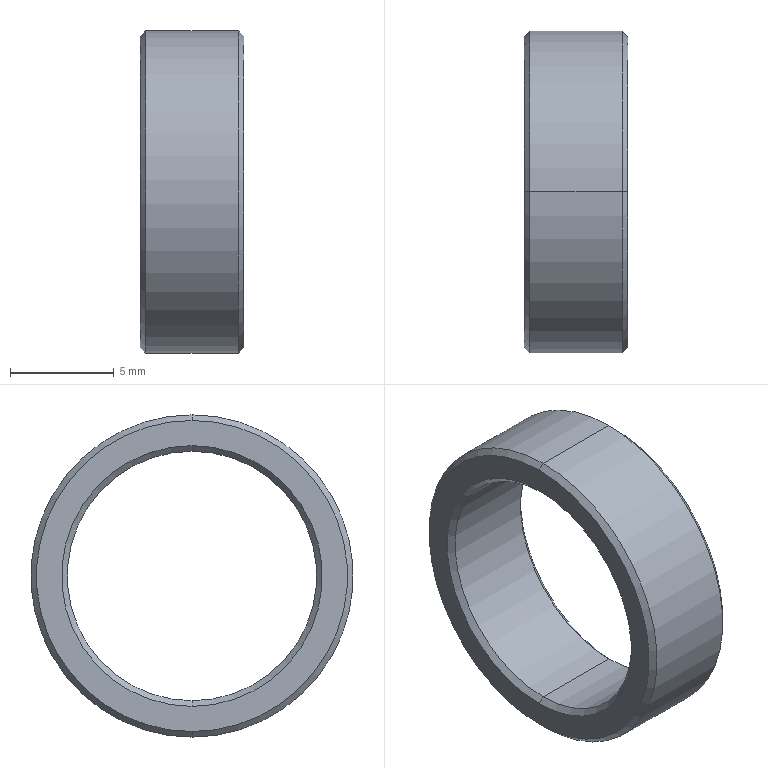Part | STEP file | GELIHUAN15-5-12-1 | 1 solid | 14 faces | box 5 x 15.5 x 15.5 mm | volume 371.674 mm3 | cone 8 | cylinder 4 | plane 2 | commonest cylinder face diameters 12 x2 15.5 x2
STEP:
#1=CARTESIAN_POINT('',(0.,0.,0.));
#2=DIRECTION('',(0.,0.,1.));
#3=DIRECTION('',(1.,0.,0.));
#4=AXIS2_PLACEMENT_3D('',#1,#2,#3);
#5=CARTESIAN_POINT('',(-8.965,58.327,-47.206));
#6=VERTEX_POINT('',#5);
#7=CARTESIAN_POINT('',(-4.505,58.327,-47.206));
#8=VERTEX_POINT('',#7);
#9=CARTESIAN_POINT('',(-8.965,58.327,-47.206));
#10=DIRECTION('',(1.,0.,0.));
#11=VECTOR('',#10,1.);
#12=LINE('',#9,#11);
#13=CARTESIAN_POINT('',(-8.965,58.327,-41.206));
#14=DIRECTION('',(1.,0.,0.));
#15=DIRECTION('',(0.,0.,-1.));
#16=AXIS2_PLACEMENT_3D('',#13,#14,#15);
#17=CYLINDRICAL_SURFACE('',#16,6.);
#18=CARTESIAN_POINT('',(6.283,0.));
#19=DIRECTION('',(0.,1.));
#20=VECTOR('',#19,1.);
#21=LINE('',#18,#20);
#22=(GEOMETRIC_REPRESENTATION_CONTEXT(2)PARAMETRIC_REPRESENTATION_CONTEXT()REPRESENTATION_CONTEXT('',''));
#23=DEFINITIONAL_REPRESENTATION('',(#21),#22);
#24=PCURVE('',#17,#23);
#25=CARTESIAN_POINT('',(-8.965,58.327,-41.206));
#26=DIRECTION('',(1.,0.,0.));
#27=DIRECTION('',(0.,0.,-1.));
#28=AXIS2_PLACEMENT_3D('',#25,#26,#27);
#29=CYLINDRICAL_SURFACE('',#28,6.);
#30=CARTESIAN_POINT('',(0.,0.));
#31=DIRECTION('',(0.,1.));
#32=VECTOR('',#31,1.);
#33=LINE('',#30,#32);
#34=(GEOMETRIC_REPRESENTATION_CONTEXT(2)PARAMETRIC_REPRESENTATION_CONTEXT()REPRESENTATION_CONTEXT('',''));
#35=DEFINITIONAL_REPRESENTATION('',(#33),#34);
#36=PCURVE('',#29,#35);
#37=SURFACE_CURVE('',#12,(#24,#36),.PCURVE_S1.);
#38=EDGE_CURVE('',#6,#8,#37,.T.);
#39=ORIENTED_EDGE('',*,*,#38,.T.);
#40=CARTESIAN_POINT('',(-4.505,58.327,-35.206));
#41=VERTEX_POINT('',#40);
#42=CARTESIAN_POINT('',(-4.505,58.327,-41.206));
#43=DIRECTION('',(-1.,0.,0.));
#44=DIRECTION('',(0.,0.,1.));
#45=AXIS2_PLACEMENT_3D('',#42,#43,#44);
#46=CIRCLE('',#45,6.);
#47=CARTESIAN_POINT('',(9.425,4.46));
#48=DIRECTION('',(-1.,0.));
#49=VECTOR('',#48,1.);
#50=LINE('',#47,#49);
#51=(GEOMETRIC_REPRESENTATION_CONTEXT(2)PARAMETRIC_REPRESENTATION_CONTEXT()REPRESENTATION_CONTEXT('',''));
#52=DEFINITIONAL_REPRESENTATION('',(#50),#51);
#53=PCURVE('',#17,#52);
#54=CARTESIAN_POINT('',(-4.505,58.327,-41.206));
#55=DIRECTION('',(1.,0.,0.));
#56=DIRECTION('',(0.,0.,-1.));
#57=AXIS2_PLACEMENT_3D('',#54,#55,#56);
#58=CONICAL_SURFACE('',#57,6.,0.7854);
#59=CARTESIAN_POINT('',(9.425,0.));
#60=DIRECTION('',(-1.,0.));
#61=VECTOR('',#60,1.);
#62=LINE('',#59,#61);
#63=(GEOMETRIC_REPRESENTATION_CONTEXT(2)PARAMETRIC_REPRESENTATION_CONTEXT()REPRESENTATION_CONTEXT('',''));
#64=DEFINITIONAL_REPRESENTATION('',(#62),#63);
#65=PCURVE('',#58,#64);
#66=SURFACE_CURVE('',#46,(#53,#65),.PCURVE_S1.);
#67=EDGE_CURVE('',#8,#41,#66,.T.);
#68=ORIENTED_EDGE('',*,*,#67,.T.);
#69=CARTESIAN_POINT('',(-8.965,58.327,-35.206));
#70=VERTEX_POINT('',#69);
#71=CARTESIAN_POINT('',(-8.965,58.327,-35.206));
#72=DIRECTION('',(1.,0.,0.));
#73=VECTOR('',#72,1.);
#74=LINE('',#71,#73);
#75=CARTESIAN_POINT('',(3.142,0.));
#76=DIRECTION('',(0.,1.));
#77=VECTOR('',#76,1.);
#78=LINE('',#75,#77);
#79=(GEOMETRIC_REPRESENTATION_CONTEXT(2)PARAMETRIC_REPRESENTATION_CONTEXT()REPRESENTATION_CONTEXT('',''));
#80=DEFINITIONAL_REPRESENTATION('',(#78),#79);
#81=PCURVE('',#17,#80);
#82=CARTESIAN_POINT('',(3.142,0.));
#83=DIRECTION('',(0.,1.));
#84=VECTOR('',#83,1.);
#85=LINE('',#82,#84);
#86=(GEOMETRIC_REPRESENTATION_CONTEXT(2)PARAMETRIC_REPRESENTATION_CONTEXT()REPRESENTATION_CONTEXT('',''));
#87=DEFINITIONAL_REPRESENTATION('',(#85),#86);
#88=PCURVE('',#29,#87);
#89=SURFACE_CURVE('',#74,(#81,#88),.PCURVE_S1.);
#90=EDGE_CURVE('',#70,#41,#89,.T.);
#91=ORIENTED_EDGE('',*,*,#90,.F.);
#92=CARTESIAN_POINT('',(-8.965,58.327,-41.206));
#93=DIRECTION('',(1.,0.,0.));
#94=DIRECTION('',(0.,0.,1.));
#95=AXIS2_PLACEMENT_3D('',#92,#93,#94);
#96=CIRCLE('',#95,6.);
#97=CARTESIAN_POINT('',(3.142,0.));
#98=DIRECTION('',(1.,0.));
#99=VECTOR('',#98,1.);
#100=LINE('',#97,#99);
#101=(GEOMETRIC_REPRESENTATION_CONTEXT(2)PARAMETRIC_REPRESENTATION_CONTEXT()REPRESENTATION_CONTEXT('',''));
#102=DEFINITIONAL_REPRESENTATION('',(#100),#101);
#103=PCURVE('',#17,#102);
#104=CARTESIAN_POINT('',(-8.965,58.327,-41.206));
#105=DIRECTION('',(-1.,0.,0.));
#106=DIRECTION('',(0.,0.,1.));
#107=AXIS2_PLACEMENT_3D('',#104,#105,#106);
#108=CONICAL_SURFACE('',#107,6.,0.7854);
#109=CARTESIAN_POINT('',(6.283,0.));
#110=DIRECTION('',(-1.,0.));
#111=VECTOR('',#110,1.);
#112=LINE('',#109,#111);
#113=(GEOMETRIC_REPRESENTATION_CONTEXT(2)PARAMETRIC_REPRESENTATION_CONTEXT()REPRESENTATION_CONTEXT('',''));
#114=DEFINITIONAL_REPRESENTATION('',(#112),#113);
#115=PCURVE('',#108,#114);
#116=SURFACE_CURVE('',#96,(#103,#115),.PCURVE_S1.);
#117=EDGE_CURVE('',#70,#6,#116,.T.);
#118=ORIENTED_EDGE('',*,*,#117,.T.);
#119=EDGE_LOOP('',(#39,#68,#91,#118));
#120=FACE_BOUND('',#119,.F.);
#121=ADVANCED_FACE('',(#120),#17,.F.);
#122=CARTESIAN_POINT('',(-9.235,58.327,-34.936));
#123=VERTEX_POINT('',#122);
#124=CARTESIAN_POINT('',(-8.965,58.327,-35.206));
#125=DIRECTION('',(-0.7071,0.,0.7071));
#126=VECTOR('',#125,1.);
#127=LINE('',#124,#126);
#128=CARTESIAN_POINT('',(6.283,0.));
#129=DIRECTION('',(0.,1.));
#130=VECTOR('',#129,1.);
#131=LINE('',#128,#130);
#132=(GEOMETRIC_REPRESENTATION_CONTEXT(2)PARAMETRIC_REPRESENTATION_CONTEXT()REPRESENTATION_CONTEXT('',''));
#133=DEFINITIONAL_REPRESENTATION('',(#131),#132);
#134=PCURVE('',#108,#133);
#135=CARTESIAN_POINT('',(-8.965,58.327,-41.206));
#136=DIRECTION('',(-1.,0.,0.));
#137=DIRECTION('',(0.,0.,1.));
#138=AXIS2_PLACEMENT_3D('',#135,#136,#137);
#139=CONICAL_SURFACE('',#138,6.,0.7854);
#140=CARTESIAN_POINT('',(0.,0.));
#141=DIRECTION('',(0.,1.));
#142=VECTOR('',#141,1.);
#143=LINE('',#140,#142);
#144=(GEOMETRIC_REPRESENTATION_CONTEXT(2)PARAMETRIC_REPRESENTATION_CONTEXT()REPRESENTATION_CONTEXT('',''));
#145=DEFINITIONAL_REPRESENTATION('',(#143),#144);
#146=PCURVE('',#139,#145);
#147=SURFACE_CURVE('',#127,(#134,#146),.PCURVE_S1.);
#148=EDGE_CURVE('',#70,#123,#147,.T.);
#149=ORIENTED_EDGE('',*,*,#148,.T.);
#150=CARTESIAN_POINT('',(-9.235,58.327,-47.476));
#151=VERTEX_POINT('',#150);
#152=CARTESIAN_POINT('',(-9.235,58.327,-41.206));
#153=DIRECTION('',(1.,0.,0.));
#154=DIRECTION('',(0.,0.,-1.));
#155=AXIS2_PLACEMENT_3D('',#152,#153,#154);
#156=CIRCLE('',#155,6.27);
#157=CARTESIAN_POINT('',(9.425,0.27));
#158=DIRECTION('',(-1.,0.));
#159=VECTOR('',#158,1.);
#160=LINE('',#157,#159);
#161=(GEOMETRIC_REPRESENTATION_CONTEXT(2)PARAMETRIC_REPRESENTATION_CONTEXT()REPRESENTATION_CONTEXT('',''));
#162=DEFINITIONAL_REPRESENTATION('',(#160),#161);
#163=PCURVE('',#108,#162);
#164=CARTESIAN_POINT('',(-9.235,66.112,-48.985));
#165=DIRECTION('',(1.,0.,0.));
#166=DIRECTION('',(0.,0.,1.));
#167=AXIS2_PLACEMENT_3D('',#164,#165,#166);
#168=PLANE('',#167);
#169=CARTESIAN_POINT('',(7.779,7.785));
#170=DIRECTION('',(-1.,0.));
#171=AXIS2_PLACEMENT_2D('',#169,#170);
#172=CIRCLE('',#171,6.27);
#173=(GEOMETRIC_REPRESENTATION_CONTEXT(2)PARAMETRIC_REPRESENTATION_CONTEXT()REPRESENTATION_CONTEXT('',''));
#174=DEFINITIONAL_REPRESENTATION('',(#172),#173);
#175=PCURVE('',#168,#174);
#176=SURFACE_CURVE('',#156,(#163,#175),.PCURVE_S1.);
#177=EDGE_CURVE('',#123,#151,#176,.T.);
#178=ORIENTED_EDGE('',*,*,#177,.T.);
#179=CARTESIAN_POINT('',(-8.965,58.327,-47.206));
#180=DIRECTION('',(-0.7071,0.,-0.7071));
#181=VECTOR('',#180,1.);
#182=LINE('',#179,#181);
#183=CARTESIAN_POINT('',(3.142,0.));
#184=DIRECTION('',(0.,1.));
#185=VECTOR('',#184,1.);
#186=LINE('',#183,#185);
#187=(GEOMETRIC_REPRESENTATION_CONTEXT(2)PARAMETRIC_REPRESENTATION_CONTEXT()REPRESENTATION_CONTEXT('',''));
#188=DEFINITIONAL_REPRESENTATION('',(#186),#187);
#189=PCURVE('',#108,#188);
#190=CARTESIAN_POINT('',(3.142,0.));
#191=DIRECTION('',(0.,1.));
#192=VECTOR('',#191,1.);
#193=LINE('',#190,#192);
#194=(GEOMETRIC_REPRESENTATION_CONTEXT(2)PARAMETRIC_REPRESENTATION_CONTEXT()REPRESENTATION_CONTEXT('',''));
#195=DEFINITIONAL_REPRESENTATION('',(#193),#194);
#196=PCURVE('',#139,#195);
#197=SURFACE_CURVE('',#182,(#189,#196),.PCURVE_S1.);
#198=EDGE_CURVE('',#6,#151,#197,.T.);
#199=ORIENTED_EDGE('',*,*,#198,.F.);
#200=ORIENTED_EDGE('',*,*,#117,.F.);
#201=EDGE_LOOP('',(#149,#178,#199,#200));
#202=FACE_BOUND('',#201,.F.);
#203=ADVANCED_FACE('',(#202),#108,.F.);
#204=CARTESIAN_POINT('',(-4.235,58.327,-47.476));
#205=VERTEX_POINT('',#204);
#206=CARTESIAN_POINT('',(-4.505,58.327,-47.206));
#207=DIRECTION('',(0.7071,0.,-0.7071));
#208=VECTOR('',#207,1.);
#209=LINE('',#206,#208);
#210=CARTESIAN_POINT('',(6.283,0.));
#211=DIRECTION('',(0.,1.));
#212=VECTOR('',#211,1.);
#213=LINE('',#210,#212);
#214=(GEOMETRIC_REPRESENTATION_CONTEXT(2)PARAMETRIC_REPRESENTATION_CONTEXT()REPRESENTATION_CONTEXT('',''));
#215=DEFINITIONAL_REPRESENTATION('',(#213),#214);
#216=PCURVE('',#58,#215);
#217=CARTESIAN_POINT('',(-4.505,58.327,-41.206));
#218=DIRECTION('',(1.,0.,0.));
#219=DIRECTION('',(0.,0.,-1.));
#220=AXIS2_PLACEMENT_3D('',#217,#218,#219);
#221=CONICAL_SURFACE('',#220,6.,0.7854);
#222=CARTESIAN_POINT('',(0.,0.));
#223=DIRECTION('',(0.,1.));
#224=VECTOR('',#223,1.);
#225=LINE('',#222,#224);
#226=(GEOMETRIC_REPRESENTATION_CONTEXT(2)PARAMETRIC_REPRESENTATION_CONTEXT()REPRESENTATION_CONTEXT('',''));
#227=DEFINITIONAL_REPRESENTATION('',(#225),#226);
#228=PCURVE('',#221,#227);
#229=SURFACE_CURVE('',#209,(#216,#228),.PCURVE_S1.);
#230=EDGE_CURVE('',#8,#205,#229,.T.);
#231=ORIENTED_EDGE('',*,*,#230,.T.);
#232=CARTESIAN_POINT('',(-4.235,58.327,-34.936));
#233=VERTEX_POINT('',#232);
#234=CARTESIAN_POINT('',(-4.235,58.327,-41.206));
#235=DIRECTION('',(-1.,0.,0.));
#236=DIRECTION('',(0.,0.,-1.));
#237=AXIS2_PLACEMENT_3D('',#234,#235,#236);
#238=CIRCLE('',#237,6.27);
#239=CARTESIAN_POINT('',(6.283,0.27));
#240=DIRECTION('',(-1.,0.));
#241=VECTOR('',#240,1.);
#242=LINE('',#239,#241);
#243=(GEOMETRIC_REPRESENTATION_CONTEXT(2)PARAMETRIC_REPRESENTATION_CONTEXT()REPRESENTATION_CONTEXT('',''));
#244=DEFINITIONAL_REPRESENTATION('',(#242),#243);
#245=PCURVE('',#58,#244);
#246=CARTESIAN_POINT('',(-4.235,66.112,-48.985));
#247=DIRECTION('',(1.,0.,0.));
#248=DIRECTION('',(0.,0.,1.));
#249=AXIS2_PLACEMENT_3D('',#246,#247,#248);
#250=PLANE('',#249);
#251=CARTESIAN_POINT('',(1.509,7.785));
#252=CARTESIAN_POINT('',(1.509,18.645));
#253=CARTESIAN_POINT('',(10.914,13.215));
#254=CARTESIAN_POINT('',(20.319,7.785));
#255=CARTESIAN_POINT('',(10.914,2.355));
#256=CARTESIAN_POINT('',(1.509,-3.075));
#257=CARTESIAN_POINT('',(1.509,7.785));
#258=(BOUNDED_CURVE()B_SPLINE_CURVE(2,(#251,#252,#253,#254,#255,#256,#257),.UNSPECIFIED.,.T.,.F.)B_SPLINE_CURVE_WITH_KNOTS((1,2,2,2,2,1),(-2.094,0.,2.094,4.189,6.283,8.378),.UNSPECIFIED.)CURVE()GEOMETRIC_REPRESENTATION_ITEM()RATIONAL_B_SPLINE_CURVE((1.,0.5,1.,0.5,1.,0.5,1.))REPRESENTATION_ITEM(''));
#259=(GEOMETRIC_REPRESENTATION_CONTEXT(2)PARAMETRIC_REPRESENTATION_CONTEXT()REPRESENTATION_CONTEXT('',''));
#260=DEFINITIONAL_REPRESENTATION('',(#258),#259);
#261=PCURVE('',#250,#260);
#262=SURFACE_CURVE('',#238,(#245,#261),.PCURVE_S1.);
#263=EDGE_CURVE('',#205,#233,#262,.T.);
#264=ORIENTED_EDGE('',*,*,#263,.T.);
#265=CARTESIAN_POINT('',(-4.505,58.327,-35.206));
#266=DIRECTION('',(0.7071,0.,0.7071));
#267=VECTOR('',#266,1.);
#268=LINE('',#265,#267);
#269=CARTESIAN_POINT('',(3.142,0.));
#270=DIRECTION('',(0.,1.));
#271=VECTOR('',#270,1.);
#272=LINE('',#269,#271);
#273=(GEOMETRIC_REPRESENTATION_CONTEXT(2)PARAMETRIC_REPRESENTATION_CONTEXT()REPRESENTATION_CONTEXT('',''));
#274=DEFINITIONAL_REPRESENTATION('',(#272),#273);
#275=PCURVE('',#58,#274);
#276=CARTESIAN_POINT('',(3.142,0.));
#277=DIRECTION('',(0.,1.));
#278=VECTOR('',#277,1.);
#279=LINE('',#276,#278);
#280=(GEOMETRIC_REPRESENTATION_CONTEXT(2)PARAMETRIC_REPRESENTATION_CONTEXT()REPRESENTATION_CONTEXT('',''));
#281=DEFINITIONAL_REPRESENTATION('',(#279),#280);
#282=PCURVE('',#221,#281);
#283=SURFACE_CURVE('',#268,(#275,#282),.PCURVE_S1.);
#284=EDGE_CURVE('',#41,#233,#283,.T.);
#285=ORIENTED_EDGE('',*,*,#284,.F.);
#286=ORIENTED_EDGE('',*,*,#67,.F.);
#287=EDGE_LOOP('',(#231,#264,#285,#286));
#288=FACE_BOUND('',#287,.F.);
#289=ADVANCED_FACE('',(#288),#58,.F.);
#290=CARTESIAN_POINT('',(-9.235,58.327,-48.686));
#291=VERTEX_POINT('',#290);
#292=CARTESIAN_POINT('',(-9.235,58.327,-33.726));
#293=VERTEX_POINT('',#292);
#294=CARTESIAN_POINT('',(-9.235,58.327,-41.206));
#295=DIRECTION('',(1.,0.,0.));
#296=DIRECTION('',(0.,0.,-1.));
#297=AXIS2_PLACEMENT_3D('',#294,#295,#296);
#298=CIRCLE('',#297,7.48);
#299=CARTESIAN_POINT('',(-9.235,58.327,-41.206));
#300=DIRECTION('',(1.,0.,0.));
#301=DIRECTION('',(0.,0.,-1.));
#302=AXIS2_PLACEMENT_3D('',#299,#300,#301);
#303=CONICAL_SURFACE('',#302,7.48,0.7854);
#304=CARTESIAN_POINT('',(0.,0.));
#305=DIRECTION('',(1.,0.));
#306=VECTOR('',#305,1.);
#307=LINE('',#304,#306);
#308=(GEOMETRIC_REPRESENTATION_CONTEXT(2)PARAMETRIC_REPRESENTATION_CONTEXT()REPRESENTATION_CONTEXT('',''));
#309=DEFINITIONAL_REPRESENTATION('',(#307),#308);
#310=PCURVE('',#303,#309);
#311=CARTESIAN_POINT('',(7.779,7.785));
#312=DIRECTION('',(-1.,0.));
#313=AXIS2_PLACEMENT_2D('',#311,#312);
#314=CIRCLE('',#313,7.48);
#315=(GEOMETRIC_REPRESENTATION_CONTEXT(2)PARAMETRIC_REPRESENTATION_CONTEXT()REPRESENTATION_CONTEXT('',''));
#316=DEFINITIONAL_REPRESENTATION('',(#314),#315);
#317=PCURVE('',#168,#316);
#318=SURFACE_CURVE('',#298,(#310,#317),.PCURVE_S1.);
#319=EDGE_CURVE('',#291,#293,#318,.T.);
#320=ORIENTED_EDGE('',*,*,#319,.T.);
#321=CARTESIAN_POINT('',(-8.965,58.327,-33.456));
#322=VERTEX_POINT('',#321);
#323=CARTESIAN_POINT('',(-9.235,58.327,-33.726));
#324=DIRECTION('',(0.7071,0.,0.7071));
#325=VECTOR('',#324,1.);
#326=LINE('',#323,#325);
#327=CARTESIAN_POINT('',(3.142,0.));
#328=DIRECTION('',(0.,1.));
#329=VECTOR('',#328,1.);
#330=LINE('',#327,#329);
#331=(GEOMETRIC_REPRESENTATION_CONTEXT(2)PARAMETRIC_REPRESENTATION_CONTEXT()REPRESENTATION_CONTEXT('',''));
#332=DEFINITIONAL_REPRESENTATION('',(#330),#331);
#333=PCURVE('',#303,#332);
#334=CARTESIAN_POINT('',(-9.235,58.327,-41.206));
#335=DIRECTION('',(1.,0.,0.));
#336=DIRECTION('',(0.,0.,-1.));
#337=AXIS2_PLACEMENT_3D('',#334,#335,#336);
#338=CONICAL_SURFACE('',#337,7.48,0.7854);
#339=CARTESIAN_POINT('',(3.142,0.));
#340=DIRECTION('',(0.,1.));
#341=VECTOR('',#340,1.);
#342=LINE('',#339,#341);
#343=(GEOMETRIC_REPRESENTATION_CONTEXT(2)PARAMETRIC_REPRESENTATION_CONTEXT()REPRESENTATION_CONTEXT('',''));
#344=DEFINITIONAL_REPRESENTATION('',(#342),#343);
#345=PCURVE('',#338,#344);
#346=SURFACE_CURVE('',#326,(#333,#345),.PCURVE_S1.);
#347=EDGE_CURVE('',#293,#322,#346,.T.);
#348=ORIENTED_EDGE('',*,*,#347,.T.);
#349=CARTESIAN_POINT('',(-8.965,58.327,-48.956));
#350=VERTEX_POINT('',#349);
#351=CARTESIAN_POINT('',(-8.965,58.327,-41.206));
#352=DIRECTION('',(1.,0.,0.));
#353=DIRECTION('',(0.,0.,-1.));
#354=AXIS2_PLACEMENT_3D('',#351,#352,#353);
#355=CIRCLE('',#354,7.75);
#356=CARTESIAN_POINT('',(0.,0.27));
#357=DIRECTION('',(1.,0.));
#358=VECTOR('',#357,1.);
#359=LINE('',#356,#358);
#360=(GEOMETRIC_REPRESENTATION_CONTEXT(2)PARAMETRIC_REPRESENTATION_CONTEXT()REPRESENTATION_CONTEXT('',''));
#361=DEFINITIONAL_REPRESENTATION('',(#359),#360);
#362=PCURVE('',#303,#361);
#363=CARTESIAN_POINT('',(-8.965,58.327,-41.206));
#364=DIRECTION('',(1.,0.,0.));
#365=DIRECTION('',(0.,0.,-1.));
#366=AXIS2_PLACEMENT_3D('',#363,#364,#365);
#367=CYLINDRICAL_SURFACE('',#366,7.75);
#368=CARTESIAN_POINT('',(0.,0.000000318));
#369=DIRECTION('',(1.,0.));
#370=VECTOR('',#369,1.);
#371=LINE('',#368,#370);
#372=(GEOMETRIC_REPRESENTATION_CONTEXT(2)PARAMETRIC_REPRESENTATION_CONTEXT()REPRESENTATION_CONTEXT('',''));
#373=DEFINITIONAL_REPRESENTATION('',(#371),#372);
#374=PCURVE('',#367,#373);
#375=SURFACE_CURVE('',#355,(#362,#374),.PCURVE_S1.);
#376=EDGE_CURVE('',#350,#322,#375,.T.);
#377=ORIENTED_EDGE('',*,*,#376,.F.);
#378=CARTESIAN_POINT('',(-9.235,58.327,-48.686));
#379=DIRECTION('',(0.7071,0.,-0.7071));
#380=VECTOR('',#379,1.);
#381=LINE('',#378,#380);
#382=CARTESIAN_POINT('',(0.,0.));
#383=DIRECTION('',(0.,1.));
#384=VECTOR('',#383,1.);
#385=LINE('',#382,#384);
#386=(GEOMETRIC_REPRESENTATION_CONTEXT(2)PARAMETRIC_REPRESENTATION_CONTEXT()REPRESENTATION_CONTEXT('',''));
#387=DEFINITIONAL_REPRESENTATION('',(#385),#386);
#388=PCURVE('',#303,#387);
#389=CARTESIAN_POINT('',(6.283,0.));
#390=DIRECTION('',(0.,1.));
#391=VECTOR('',#390,1.);
#392=LINE('',#389,#391);
#393=(GEOMETRIC_REPRESENTATION_CONTEXT(2)PARAMETRIC_REPRESENTATION_CONTEXT()REPRESENTATION_CONTEXT('',''));
#394=DEFINITIONAL_REPRESENTATION('',(#392),#393);
#395=PCURVE('',#338,#394);
#396=SURFACE_CURVE('',#381,(#388,#395),.PCURVE_S1.);
#397=EDGE_CURVE('',#291,#350,#396,.T.);
#398=ORIENTED_EDGE('',*,*,#397,.F.);
#399=EDGE_LOOP('',(#320,#348,#377,#398));
#400=FACE_BOUND('',#399,.T.);
#401=ADVANCED_FACE('',(#400),#303,.T.);
#402=CARTESIAN_POINT('',(-4.235,58.327,-33.726));
#403=VERTEX_POINT('',#402);
#404=CARTESIAN_POINT('',(-4.235,58.327,-48.686));
#405=VERTEX_POINT('',#404);
#406=CARTESIAN_POINT('',(-4.235,58.327,-41.206));
#407=DIRECTION('',(-1.,0.,0.));
#408=DIRECTION('',(0.,0.,1.));
#409=AXIS2_PLACEMENT_3D('',#406,#407,#408);
#410=CIRCLE('',#409,7.48);
#411=CARTESIAN_POINT('',(-4.235,58.327,-41.206));
#412=DIRECTION('',(-1.,0.,0.));
#413=DIRECTION('',(0.,0.,1.));
#414=AXIS2_PLACEMENT_3D('',#411,#412,#413);
#415=CONICAL_SURFACE('',#414,7.48,0.7854);
#416=CARTESIAN_POINT('',(0.,0.));
#417=DIRECTION('',(1.,0.));
#418=VECTOR('',#417,1.);
#419=LINE('',#416,#418);
#420=(GEOMETRIC_REPRESENTATION_CONTEXT(2)PARAMETRIC_REPRESENTATION_CONTEXT()REPRESENTATION_CONTEXT('',''));
#421=DEFINITIONAL_REPRESENTATION('',(#419),#420);
#422=PCURVE('',#415,#421);
#423=CARTESIAN_POINT('',(15.259,7.785));
#424=CARTESIAN_POINT('',(15.259,-5.171));
#425=CARTESIAN_POINT('',(4.039,1.307));
#426=CARTESIAN_POINT('',(-7.181,7.785));
#427=CARTESIAN_POINT('',(4.039,14.262));
#428=CARTESIAN_POINT('',(15.259,20.74));
#429=CARTESIAN_POINT('',(15.259,7.785));
#430=(BOUNDED_CURVE()B_SPLINE_CURVE(2,(#423,#424,#425,#426,#427,#428,#429),.UNSPECIFIED.,.T.,.F.)B_SPLINE_CURVE_WITH_KNOTS((1,2,2,2,2,1),(-2.094,0.,2.094,4.189,6.283,8.378),.UNSPECIFIED.)CURVE()GEOMETRIC_REPRESENTATION_ITEM()RATIONAL_B_SPLINE_CURVE((1.,0.5,1.,0.5,1.,0.5,1.))REPRESENTATION_ITEM(''));
#431=(GEOMETRIC_REPRESENTATION_CONTEXT(2)PARAMETRIC_REPRESENTATION_CONTEXT()REPRESENTATION_CONTEXT('',''));
#432=DEFINITIONAL_REPRESENTATION('',(#430),#431);
#433=PCURVE('',#250,#432);
#434=SURFACE_CURVE('',#410,(#422,#433),.PCURVE_S1.);
#435=EDGE_CURVE('',#403,#405,#434,.T.);
#436=ORIENTED_EDGE('',*,*,#435,.T.);
#437=CARTESIAN_POINT('',(-4.505,58.327,-48.956));
#438=VERTEX_POINT('',#437);
#439=CARTESIAN_POINT('',(-4.235,58.327,-48.686));
#440=DIRECTION('',(-0.7071,0.,-0.7071));
#441=VECTOR('',#440,1.);
#442=LINE('',#439,#441);
#443=CARTESIAN_POINT('',(3.142,0.));
#444=DIRECTION('',(0.,1.));
#445=VECTOR('',#444,1.);
#446=LINE('',#443,#445);
#447=(GEOMETRIC_REPRESENTATION_CONTEXT(2)PARAMETRIC_REPRESENTATION_CONTEXT()REPRESENTATION_CONTEXT('',''));
#448=DEFINITIONAL_REPRESENTATION('',(#446),#447);
#449=PCURVE('',#415,#448);
#450=CARTESIAN_POINT('',(-4.235,58.327,-41.206));
#451=DIRECTION('',(-1.,0.,0.));
#452=DIRECTION('',(0.,0.,1.));
#453=AXIS2_PLACEMENT_3D('',#450,#451,#452);
#454=CONICAL_SURFACE('',#453,7.48,0.7854);
#455=CARTESIAN_POINT('',(3.142,0.));
#456=DIRECTION('',(0.,1.));
#457=VECTOR('',#456,1.);
#458=LINE('',#455,#457);
#459=(GEOMETRIC_REPRESENTATION_CONTEXT(2)PARAMETRIC_REPRESENTATION_CONTEXT()REPRESENTATION_CONTEXT('',''));
#460=DEFINITIONAL_REPRESENTATION('',(#458),#459);
#461=PCURVE('',#454,#460);
#462=SURFACE_CURVE('',#442,(#449,#461),.PCURVE_S1.);
#463=EDGE_CURVE('',#405,#438,#462,.T.);
#464=ORIENTED_EDGE('',*,*,#463,.T.);
#465=CARTESIAN_POINT('',(-4.505,58.327,-33.456));
#466=VERTEX_POINT('',#465);
#467=CARTESIAN_POINT('',(-4.505,58.327,-41.206));
#468=DIRECTION('',(-1.,0.,0.));
#469=DIRECTION('',(0.,0.,-1.));
#470=AXIS2_PLACEMENT_3D('',#467,#468,#469);
#471=CIRCLE('',#470,7.75);
#472=CARTESIAN_POINT('',(-3.142,0.27));
#473=DIRECTION('',(1.,0.));
#474=VECTOR('',#473,1.);
#475=LINE('',#472,#474);
#476=(GEOMETRIC_REPRESENTATION_CONTEXT(2)PARAMETRIC_REPRESENTATION_CONTEXT()REPRESENTATION_CONTEXT('',''));
#477=DEFINITIONAL_REPRESENTATION('',(#475),#476);
#478=PCURVE('',#415,#477);
#479=CARTESIAN_POINT('',(6.283,4.46));
#480=DIRECTION('',(-1.,0.));
#481=VECTOR('',#480,1.);
#482=LINE('',#479,#481);
#483=(GEOMETRIC_REPRESENTATION_CONTEXT(2)PARAMETRIC_REPRESENTATION_CONTEXT()REPRESENTATION_CONTEXT('',''));
#484=DEFINITIONAL_REPRESENTATION('',(#482),#483);
#485=PCURVE('',#367,#484);
#486=SURFACE_CURVE('',#471,(#478,#485),.PCURVE_S1.);
#487=EDGE_CURVE('',#466,#438,#486,.T.);
#488=ORIENTED_EDGE('',*,*,#487,.F.);
#489=CARTESIAN_POINT('',(-4.235,58.327,-33.726));
#490=DIRECTION('',(-0.7071,0.,0.7071));
#491=VECTOR('',#490,1.);
#492=LINE('',#489,#491);
#493=CARTESIAN_POINT('',(0.,0.));
#494=DIRECTION('',(0.,1.));
#495=VECTOR('',#494,1.);
#496=LINE('',#493,#495);
#497=(GEOMETRIC_REPRESENTATION_CONTEXT(2)PARAMETRIC_REPRESENTATION_CONTEXT()REPRESENTATION_CONTEXT('',''));
#498=DEFINITIONAL_REPRESENTATION('',(#496),#497);
#499=PCURVE('',#415,#498);
#500=CARTESIAN_POINT('',(6.283,0.));
#501=DIRECTION('',(0.,1.));
#502=VECTOR('',#501,1.);
#503=LINE('',#500,#502);
#504=(GEOMETRIC_REPRESENTATION_CONTEXT(2)PARAMETRIC_REPRESENTATION_CONTEXT()REPRESENTATION_CONTEXT('',''));
#505=DEFINITIONAL_REPRESENTATION('',(#503),#504);
#506=PCURVE('',#454,#505);
#507=SURFACE_CURVE('',#492,(#499,#506),.PCURVE_S1.);
#508=EDGE_CURVE('',#403,#466,#507,.T.);
#509=ORIENTED_EDGE('',*,*,#508,.F.);
#510=EDGE_LOOP('',(#436,#464,#488,#509));
#511=FACE_BOUND('',#510,.T.);
#512=ADVANCED_FACE('',(#511),#415,.T.);
#513=ORIENTED_EDGE('',*,*,#376,.T.);
#514=CARTESIAN_POINT('',(-8.965,58.327,-33.456));
#515=DIRECTION('',(1.,0.,0.));
#516=VECTOR('',#515,1.);
#517=LINE('',#514,#516);
#518=CARTESIAN_POINT('',(3.142,0.));
#519=DIRECTION('',(0.,1.));
#520=VECTOR('',#519,1.);
#521=LINE('',#518,#520);
#522=(GEOMETRIC_REPRESENTATION_CONTEXT(2)PARAMETRIC_REPRESENTATION_CONTEXT()REPRESENTATION_CONTEXT('',''));
#523=DEFINITIONAL_REPRESENTATION('',(#521),#522);
#524=PCURVE('',#367,#523);
#525=CARTESIAN_POINT('',(-8.965,58.327,-41.206));
#526=DIRECTION('',(1.,0.,0.));
#527=DIRECTION('',(0.,0.,-1.));
#528=AXIS2_PLACEMENT_3D('',#525,#526,#527);
#529=CYLINDRICAL_SURFACE('',#528,7.75);
#530=CARTESIAN_POINT('',(3.142,0.));
#531=DIRECTION('',(0.,1.));
#532=VECTOR('',#531,1.);
#533=LINE('',#530,#532);
#534=(GEOMETRIC_REPRESENTATION_CONTEXT(2)PARAMETRIC_REPRESENTATION_CONTEXT()REPRESENTATION_CONTEXT('',''));
#535=DEFINITIONAL_REPRESENTATION('',(#533),#534);
#536=PCURVE('',#529,#535);
#537=SURFACE_CURVE('',#517,(#524,#536),.PCURVE_S1.);
#538=EDGE_CURVE('',#322,#466,#537,.T.);
#539=ORIENTED_EDGE('',*,*,#538,.T.);
#540=ORIENTED_EDGE('',*,*,#487,.T.);
#541=CARTESIAN_POINT('',(-8.965,58.327,-48.956));
#542=DIRECTION('',(1.,0.,0.));
#543=VECTOR('',#542,1.);
#544=LINE('',#541,#543);
#545=CARTESIAN_POINT('',(0.,0.));
#546=DIRECTION('',(0.,1.));
#547=VECTOR('',#546,1.);
#548=LINE('',#545,#547);
#549=(GEOMETRIC_REPRESENTATION_CONTEXT(2)PARAMETRIC_REPRESENTATION_CONTEXT()REPRESENTATION_CONTEXT('',''));
#550=DEFINITIONAL_REPRESENTATION('',(#548),#549);
#551=PCURVE('',#367,#550);
#552=CARTESIAN_POINT('',(6.283,0.));
#553=DIRECTION('',(0.,1.));
#554=VECTOR('',#553,1.);
#555=LINE('',#552,#554);
#556=(GEOMETRIC_REPRESENTATION_CONTEXT(2)PARAMETRIC_REPRESENTATION_CONTEXT()REPRESENTATION_CONTEXT('',''));
#557=DEFINITIONAL_REPRESENTATION('',(#555),#556);
#558=PCURVE('',#529,#557);
#559=SURFACE_CURVE('',#544,(#551,#558),.PCURVE_S1.);
#560=EDGE_CURVE('',#350,#438,#559,.T.);
#561=ORIENTED_EDGE('',*,*,#560,.F.);
#562=EDGE_LOOP('',(#513,#539,#540,#561));
#563=FACE_BOUND('',#562,.T.);
#564=ADVANCED_FACE('',(#563),#367,.T.);
#565=CARTESIAN_POINT('',(-4.505,58.327,-41.206));
#566=DIRECTION('',(-1.,0.,0.));
#567=DIRECTION('',(0.,0.,1.));
#568=AXIS2_PLACEMENT_3D('',#565,#566,#567);
#569=CIRCLE('',#568,6.);
#570=CARTESIAN_POINT('',(3.142,4.46));
#571=DIRECTION('',(-1.,0.));
#572=VECTOR('',#571,1.);
#573=LINE('',#570,#572);
#574=(GEOMETRIC_REPRESENTATION_CONTEXT(2)PARAMETRIC_REPRESENTATION_CONTEXT()REPRESENTATION_CONTEXT('',''));
#575=DEFINITIONAL_REPRESENTATION('',(#573),#574);
#576=PCURVE('',#29,#575);
#577=CARTESIAN_POINT('',(3.142,0.));
#578=DIRECTION('',(-1.,0.));
#579=VECTOR('',#578,1.);
#580=LINE('',#577,#579);
#581=(GEOMETRIC_REPRESENTATION_CONTEXT(2)PARAMETRIC_REPRESENTATION_CONTEXT()REPRESENTATION_CONTEXT('',''));
#582=DEFINITIONAL_REPRESENTATION('',(#580),#581);
#583=PCURVE('',#221,#582);
#584=SURFACE_CURVE('',#569,(#576,#583),.PCURVE_S1.);
#585=EDGE_CURVE('',#41,#8,#584,.T.);
#586=ORIENTED_EDGE('',*,*,#585,.T.);
#587=ORIENTED_EDGE('',*,*,#38,.F.);
#588=CARTESIAN_POINT('',(-8.965,58.327,-41.206));
#589=DIRECTION('',(1.,0.,0.));
#590=DIRECTION('',(0.,0.,1.));
#591=AXIS2_PLACEMENT_3D('',#588,#589,#590);
#592=CIRCLE('',#591,6.);
#593=CARTESIAN_POINT('',(-3.142,0.));
#594=DIRECTION('',(1.,0.));
#595=VECTOR('',#594,1.);
#596=LINE('',#593,#595);
#597=(GEOMETRIC_REPRESENTATION_CONTEXT(2)PARAMETRIC_REPRESENTATION_CONTEXT()REPRESENTATION_CONTEXT('',''));
#598=DEFINITIONAL_REPRESENTATION('',(#596),#597);
#599=PCURVE('',#29,#598);
#600=CARTESIAN_POINT('',(6.283,0.));
#601=DIRECTION('',(-1.,0.));
#602=VECTOR('',#601,1.);
#603=LINE('',#600,#602);
#604=(GEOMETRIC_REPRESENTATION_CONTEXT(2)PARAMETRIC_REPRESENTATION_CONTEXT()REPRESENTATION_CONTEXT('',''));
#605=DEFINITIONAL_REPRESENTATION('',(#603),#604);
#606=PCURVE('',#139,#605);
#607=SURFACE_CURVE('',#592,(#599,#606),.PCURVE_S1.);
#608=EDGE_CURVE('',#6,#70,#607,.T.);
#609=ORIENTED_EDGE('',*,*,#608,.T.);
#610=ORIENTED_EDGE('',*,*,#90,.T.);
#611=EDGE_LOOP('',(#586,#587,#609,#610));
#612=FACE_BOUND('',#611,.F.);
#613=ADVANCED_FACE('',(#612),#29,.F.);
#614=CARTESIAN_POINT('',(-9.235,58.327,-41.206));
#615=DIRECTION('',(1.,0.,0.));
#616=DIRECTION('',(0.,0.,-1.));
#617=AXIS2_PLACEMENT_3D('',#614,#615,#616);
#618=CIRCLE('',#617,6.27);
#619=CARTESIAN_POINT('',(3.142,0.27));
#620=DIRECTION('',(-1.,0.));
#621=VECTOR('',#620,1.);
#622=LINE('',#619,#621);
#623=(GEOMETRIC_REPRESENTATION_CONTEXT(2)PARAMETRIC_REPRESENTATION_CONTEXT()REPRESENTATION_CONTEXT('',''));
#624=DEFINITIONAL_REPRESENTATION('',(#622),#623);
#625=PCURVE('',#139,#624);
#626=CARTESIAN_POINT('',(7.779,7.785));
#627=DIRECTION('',(-1.,0.));
#628=AXIS2_PLACEMENT_2D('',#626,#627);
#629=CIRCLE('',#628,6.27);
#630=(GEOMETRIC_REPRESENTATION_CONTEXT(2)PARAMETRIC_REPRESENTATION_CONTEXT()REPRESENTATION_CONTEXT('',''));
#631=DEFINITIONAL_REPRESENTATION('',(#629),#630);
#632=PCURVE('',#168,#631);
#633=SURFACE_CURVE('',#618,(#625,#632),.PCURVE_S1.);
#634=EDGE_CURVE('',#151,#123,#633,.T.);
#635=ORIENTED_EDGE('',*,*,#634,.T.);
#636=ORIENTED_EDGE('',*,*,#148,.F.);
#637=ORIENTED_EDGE('',*,*,#608,.F.);
#638=ORIENTED_EDGE('',*,*,#198,.T.);
#639=EDGE_LOOP('',(#635,#636,#637,#638));
#640=FACE_BOUND('',#639,.F.);
#641=ADVANCED_FACE('',(#640),#139,.F.);
#642=CARTESIAN_POINT('',(-4.235,58.327,-41.206));
#643=DIRECTION('',(-1.,0.,0.));
#644=DIRECTION('',(0.,0.,-1.));
#645=AXIS2_PLACEMENT_3D('',#642,#643,#644);
#646=CIRCLE('',#645,6.27);
#647=CARTESIAN_POINT('',(6.283,0.27));
#648=DIRECTION('',(-1.,0.));
#649=VECTOR('',#648,1.);
#650=LINE('',#647,#649);
#651=(GEOMETRIC_REPRESENTATION_CONTEXT(2)PARAMETRIC_REPRESENTATION_CONTEXT()REPRESENTATION_CONTEXT('',''));
#652=DEFINITIONAL_REPRESENTATION('',(#650),#651);
#653=PCURVE('',#221,#652);
#654=CARTESIAN_POINT('',(1.509,7.785));
#655=CARTESIAN_POINT('',(1.509,18.645));
#656=CARTESIAN_POINT('',(10.914,13.215));
#657=CARTESIAN_POINT('',(20.319,7.785));
#658=CARTESIAN_POINT('',(10.914,2.355));
#659=CARTESIAN_POINT('',(1.509,-3.075));
#660=CARTESIAN_POINT('',(1.509,7.785));
#661=(BOUNDED_CURVE()B_SPLINE_CURVE(2,(#654,#655,#656,#657,#658,#659,#660),.UNSPECIFIED.,.T.,.F.)B_SPLINE_CURVE_WITH_KNOTS((1,2,2,2,2,1),(-2.094,0.,2.094,4.189,6.283,8.378),.UNSPECIFIED.)CURVE()GEOMETRIC_REPRESENTATION_ITEM()RATIONAL_B_SPLINE_CURVE((1.,0.5,1.,0.5,1.,0.5,1.))REPRESENTATION_ITEM(''));
#662=(GEOMETRIC_REPRESENTATION_CONTEXT(2)PARAMETRIC_REPRESENTATION_CONTEXT()REPRESENTATION_CONTEXT('',''));
#663=DEFINITIONAL_REPRESENTATION('',(#661),#662);
#664=PCURVE('',#250,#663);
#665=SURFACE_CURVE('',#646,(#653,#664),.PCURVE_S1.);
#666=EDGE_CURVE('',#233,#205,#665,.T.);
#667=ORIENTED_EDGE('',*,*,#666,.T.);
#668=ORIENTED_EDGE('',*,*,#230,.F.);
#669=ORIENTED_EDGE('',*,*,#585,.F.);
#670=ORIENTED_EDGE('',*,*,#284,.T.);
#671=EDGE_LOOP('',(#667,#668,#669,#670));
#672=FACE_BOUND('',#671,.F.);
#673=ADVANCED_FACE('',(#672),#221,.F.);
#674=ORIENTED_EDGE('',*,*,#177,.T.);
#675=ORIENTED_EDGE('',*,*,#634,.T.);
#676=EDGE_LOOP('',(#674,#675));
#677=FACE_BOUND('',#676,.T.);
#678=CARTESIAN_POINT('',(-9.235,58.327,-41.206));
#679=DIRECTION('',(1.,0.,0.));
#680=DIRECTION('',(0.,0.,-1.));
#681=AXIS2_PLACEMENT_3D('',#678,#679,#680);
#682=CIRCLE('',#681,7.48);
#683=CARTESIAN_POINT('',(7.779,7.785));
#684=DIRECTION('',(-1.,0.));
#685=AXIS2_PLACEMENT_2D('',#683,#684);
#686=CIRCLE('',#685,7.48);
#687=(GEOMETRIC_REPRESENTATION_CONTEXT(2)PARAMETRIC_REPRESENTATION_CONTEXT()REPRESENTATION_CONTEXT('',''));
#688=DEFINITIONAL_REPRESENTATION('',(#686),#687);
#689=PCURVE('',#168,#688);
#690=CARTESIAN_POINT('',(0.,0.));
#691=DIRECTION('',(1.,0.));
#692=VECTOR('',#691,1.);
#693=LINE('',#690,#692);
#694=(GEOMETRIC_REPRESENTATION_CONTEXT(2)PARAMETRIC_REPRESENTATION_CONTEXT()REPRESENTATION_CONTEXT('',''));
#695=DEFINITIONAL_REPRESENTATION('',(#693),#694);
#696=PCURVE('',#338,#695);
#697=SURFACE_CURVE('',#682,(#689,#696),.PCURVE_S1.);
#698=EDGE_CURVE('',#293,#291,#697,.T.);
#699=ORIENTED_EDGE('',*,*,#698,.T.);
#700=ORIENTED_EDGE('',*,*,#319,.T.);
#701=EDGE_LOOP('',(#699,#700));
#702=FACE_BOUND('',#701,.F.);
#703=ADVANCED_FACE('',(#677,#702),#168,.F.);
#704=ORIENTED_EDGE('',*,*,#263,.T.);
#705=ORIENTED_EDGE('',*,*,#666,.T.);
#706=EDGE_LOOP('',(#704,#705));
#707=FACE_BOUND('',#706,.T.);
#708=ORIENTED_EDGE('',*,*,#435,.F.);
#709=CARTESIAN_POINT('',(-4.235,58.327,-41.206));
#710=DIRECTION('',(-1.,0.,0.));
#711=DIRECTION('',(0.,0.,1.));
#712=AXIS2_PLACEMENT_3D('',#709,#710,#711);
#713=CIRCLE('',#712,7.48);
#714=CARTESIAN_POINT('',(15.259,7.785));
#715=CARTESIAN_POINT('',(15.259,-5.171));
#716=CARTESIAN_POINT('',(4.039,1.307));
#717=CARTESIAN_POINT('',(-7.181,7.785));
#718=CARTESIAN_POINT('',(4.039,14.262));
#719=CARTESIAN_POINT('',(15.259,20.74));
#720=CARTESIAN_POINT('',(15.259,7.785));
#721=(BOUNDED_CURVE()B_SPLINE_CURVE(2,(#714,#715,#716,#717,#718,#719,#720),.UNSPECIFIED.,.T.,.F.)B_SPLINE_CURVE_WITH_KNOTS((1,2,2,2,2,1),(-2.094,0.,2.094,4.189,6.283,8.378),.UNSPECIFIED.)CURVE()GEOMETRIC_REPRESENTATION_ITEM()RATIONAL_B_SPLINE_CURVE((1.,0.5,1.,0.5,1.,0.5,1.))REPRESENTATION_ITEM(''));
#722=(GEOMETRIC_REPRESENTATION_CONTEXT(2)PARAMETRIC_REPRESENTATION_CONTEXT()REPRESENTATION_CONTEXT('',''));
#723=DEFINITIONAL_REPRESENTATION('',(#721),#722);
#724=PCURVE('',#250,#723);
#725=CARTESIAN_POINT('',(0.,0.));
#726=DIRECTION('',(1.,0.));
#727=VECTOR('',#726,1.);
#728=LINE('',#725,#727);
#729=(GEOMETRIC_REPRESENTATION_CONTEXT(2)PARAMETRIC_REPRESENTATION_CONTEXT()REPRESENTATION_CONTEXT('',''));
#730=DEFINITIONAL_REPRESENTATION('',(#728),#729);
#731=PCURVE('',#454,#730);
#732=SURFACE_CURVE('',#713,(#724,#731),.PCURVE_S1.);
#733=EDGE_CURVE('',#405,#403,#732,.T.);
#734=ORIENTED_EDGE('',*,*,#733,.F.);
#735=EDGE_LOOP('',(#708,#734));
#736=FACE_BOUND('',#735,.T.);
#737=ADVANCED_FACE('',(#707,#736),#250,.T.);
#738=ORIENTED_EDGE('',*,*,#347,.F.);
#739=ORIENTED_EDGE('',*,*,#698,.T.);
#740=ORIENTED_EDGE('',*,*,#397,.T.);
#741=CARTESIAN_POINT('',(-8.965,58.327,-41.206));
#742=DIRECTION('',(1.,0.,0.));
#743=DIRECTION('',(0.,0.,-1.));
#744=AXIS2_PLACEMENT_3D('',#741,#742,#743);
#745=CIRCLE('',#744,7.75);
#746=CARTESIAN_POINT('',(0.,0.27));
#747=DIRECTION('',(1.,0.));
#748=VECTOR('',#747,1.);
#749=LINE('',#746,#748);
#750=(GEOMETRIC_REPRESENTATION_CONTEXT(2)PARAMETRIC_REPRESENTATION_CONTEXT()REPRESENTATION_CONTEXT('',''));
#751=DEFINITIONAL_REPRESENTATION('',(#749),#750);
#752=PCURVE('',#338,#751);
#753=CARTESIAN_POINT('',(0.,0.000000318));
#754=DIRECTION('',(1.,0.));
#755=VECTOR('',#754,1.);
#756=LINE('',#753,#755);
#757=(GEOMETRIC_REPRESENTATION_CONTEXT(2)PARAMETRIC_REPRESENTATION_CONTEXT()REPRESENTATION_CONTEXT('',''));
#758=DEFINITIONAL_REPRESENTATION('',(#756),#757);
#759=PCURVE('',#529,#758);
#760=SURFACE_CURVE('',#745,(#752,#759),.PCURVE_S1.);
#761=EDGE_CURVE('',#322,#350,#760,.T.);
#762=ORIENTED_EDGE('',*,*,#761,.F.);
#763=EDGE_LOOP('',(#738,#739,#740,#762));
#764=FACE_BOUND('',#763,.T.);
#765=ADVANCED_FACE('',(#764),#338,.T.);
#766=ORIENTED_EDGE('',*,*,#463,.F.);
#767=ORIENTED_EDGE('',*,*,#733,.T.);
#768=ORIENTED_EDGE('',*,*,#508,.T.);
#769=CARTESIAN_POINT('',(-4.505,58.327,-41.206));
#770=DIRECTION('',(-1.,0.,0.));
#771=DIRECTION('',(0.,0.,-1.));
#772=AXIS2_PLACEMENT_3D('',#769,#770,#771);
#773=CIRCLE('',#772,7.75);
#774=CARTESIAN_POINT('',(3.142,0.27));
#775=DIRECTION('',(1.,0.));
#776=VECTOR('',#775,1.);
#777=LINE('',#774,#776);
#778=(GEOMETRIC_REPRESENTATION_CONTEXT(2)PARAMETRIC_REPRESENTATION_CONTEXT()REPRESENTATION_CONTEXT('',''));
#779=DEFINITIONAL_REPRESENTATION('',(#777),#778);
#780=PCURVE('',#454,#779);
#781=CARTESIAN_POINT('',(6.283,4.46));
#782=DIRECTION('',(-1.,0.));
#783=VECTOR('',#782,1.);
#784=LINE('',#781,#783);
#785=(GEOMETRIC_REPRESENTATION_CONTEXT(2)PARAMETRIC_REPRESENTATION_CONTEXT()REPRESENTATION_CONTEXT('',''));
#786=DEFINITIONAL_REPRESENTATION('',(#784),#785);
#787=PCURVE('',#529,#786);
#788=SURFACE_CURVE('',#773,(#780,#787),.PCURVE_S1.);
#789=EDGE_CURVE('',#438,#466,#788,.T.);
#790=ORIENTED_EDGE('',*,*,#789,.F.);
#791=EDGE_LOOP('',(#766,#767,#768,#790));
#792=FACE_BOUND('',#791,.T.);
#793=ADVANCED_FACE('',(#792),#454,.T.);
#794=ORIENTED_EDGE('',*,*,#538,.F.);
#795=ORIENTED_EDGE('',*,*,#761,.T.);
#796=ORIENTED_EDGE('',*,*,#560,.T.);
#797=ORIENTED_EDGE('',*,*,#789,.T.);
#798=EDGE_LOOP('',(#794,#795,#796,#797));
#799=FACE_BOUND('',#798,.T.);
#800=ADVANCED_FACE('',(#799),#529,.T.);
#801=CLOSED_SHELL('',(#121,#203,#289,#401,#512,#564,#613,#641,#673,#703,#737,#765,#793,#800));
#802=MANIFOLD_SOLID_BREP('',#801);
#803=(LENGTH_UNIT()NAMED_UNIT(*)SI_UNIT(.MILLI.,.METRE.));
#804=UNCERTAINTY_MEASURE_WITH_UNIT(LENGTH_MEASURE(0.0000005),#803,'','');
#805=(NAMED_UNIT(*)PLANE_ANGLE_UNIT()SI_UNIT($,.RADIAN.));
#806=(NAMED_UNIT(*)SI_UNIT($,.STERADIAN.)SOLID_ANGLE_UNIT());
#807=(GEOMETRIC_REPRESENTATION_CONTEXT(3)GLOBAL_UNCERTAINTY_ASSIGNED_CONTEXT((#804))GLOBAL_UNIT_ASSIGNED_CONTEXT((#803,#805,#806))REPRESENTATION_CONTEXT('',''));
#808=ADVANCED_BREP_SHAPE_REPRESENTATION('',(#4,#802),#807);